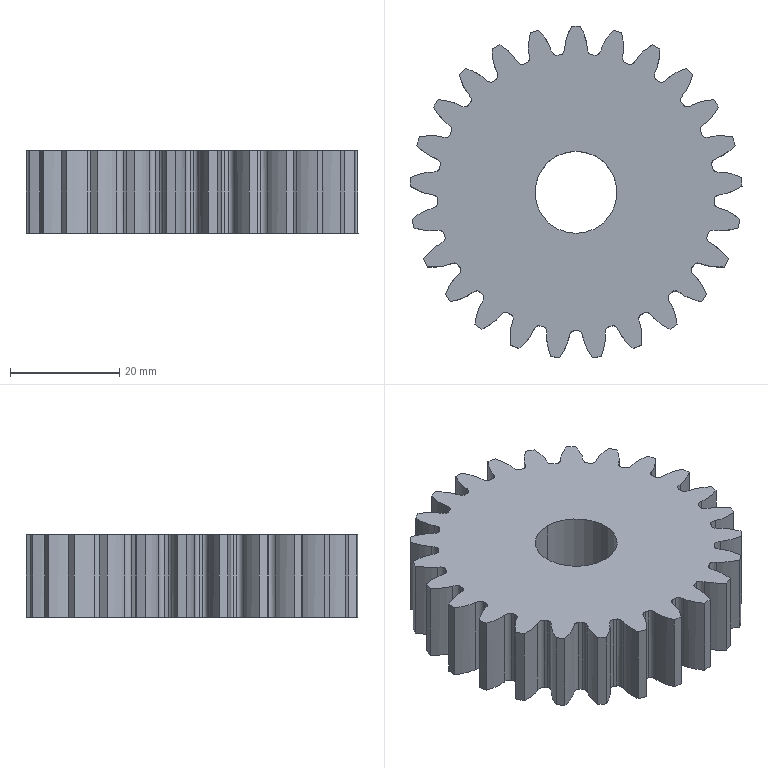Part | SolidWorks | features BaseBody 1 | 1 solid | 154 faces | box 60.71 x 60.601 x 15 mm | volume 34143 mm3 | spline 125 | cylinder 27 | plane 2 | commonest cylinder face diameters 50.625 x25 15 x2